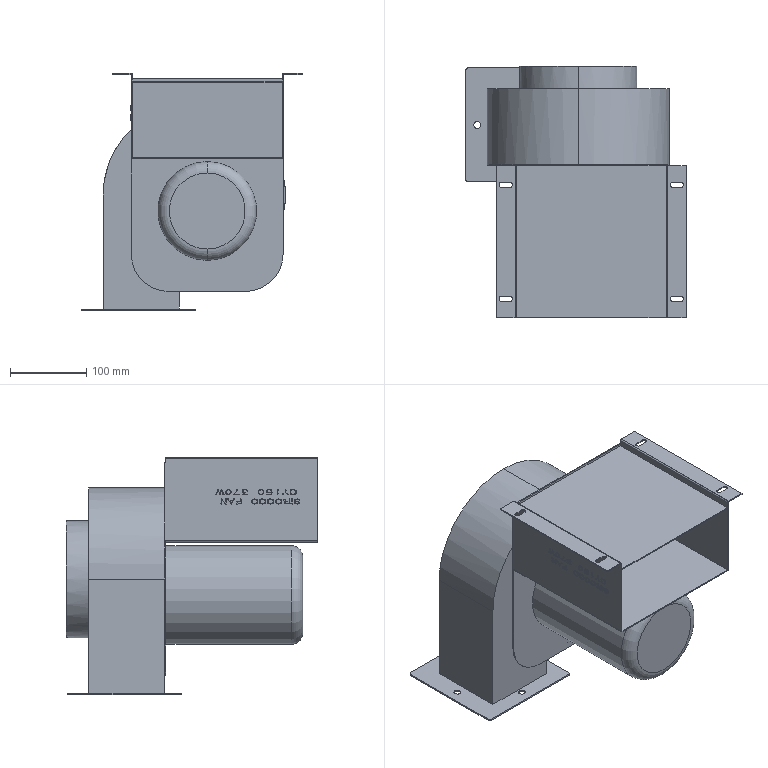Part | SolidWorks | features ICE 9, Fillet 2, SMBaseFlange 2, SheetMetal 2, FlatPattern 1, Shell 1 | 1 solid | 735 faces | box 290.055 x 331.5 x 312 mm | volume 759476 mm3 | plane 395 | cylinder 169 | spline 167 | torus 4 | commonest cylinder face diameters 4 x116 6.5 x12 9 x8 0.4 x4 3.4 x4 6 x4